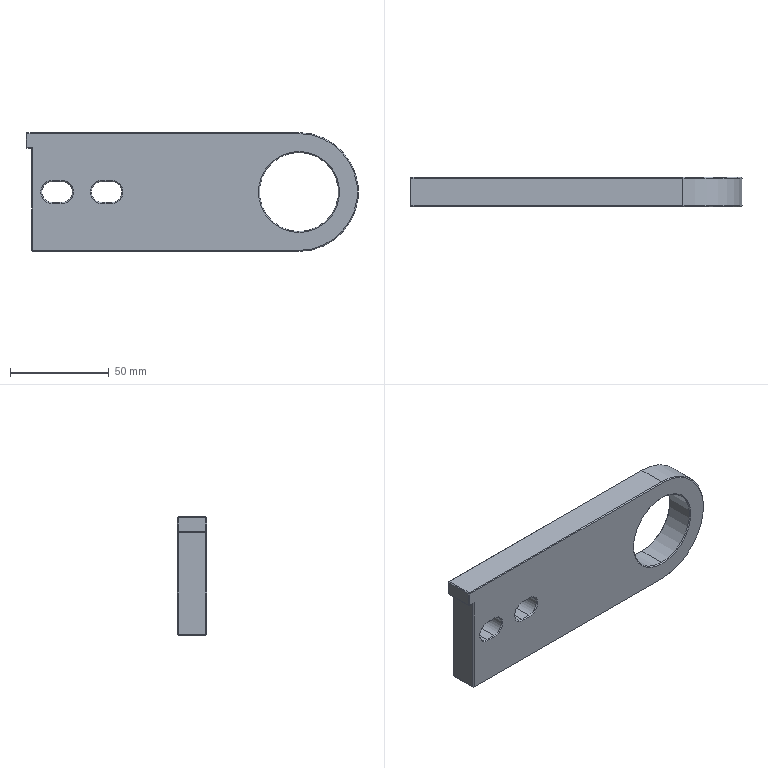Part | SolidWorks | features Chamfer 1, Extrusion 1, ICE 1 | 1 solid | 59 faces | box 168 x 15 x 60 mm | volume 119877 mm3 | plane 38 | cone 14 | cylinder 7 | commonest cylinder face diameters 10.5 x4 40 x2 60 x1
STEP:
#1=CARTESIAN_POINT('',(0.,0.5,20.));
#2=VERTEX_POINT('',#1);
#3=CARTESIAN_POINT('',(0.,0.5,-20.));
#4=VERTEX_POINT('',#3);
#5=CARTESIAN_POINT('',(0.,0.5,0.));
#6=DIRECTION('',(0.,-1.,0.));
#7=DIRECTION('',(0.,0.,1.));
#8=AXIS2_PLACEMENT_3D('',#5,#6,#7);
#9=CIRCLE('',#8,20.);
#10=EDGE_CURVE('',#2,#4,#9,.T.);
#11=ORIENTED_EDGE('',*,*,#10,.F.);
#12=CARTESIAN_POINT('',(0.,0.,20.5));
#13=VERTEX_POINT('',#12);
#14=CARTESIAN_POINT('',(0.,0.,20.5));
#15=DIRECTION('',(0.,-0.7071,0.7071));
#16=VECTOR('',#15,1000.);
#17=LINE('',#14,#16);
#18=EDGE_CURVE('',#2,#13,#17,.T.);
#19=ORIENTED_EDGE('',*,*,#18,.T.);
#20=CARTESIAN_POINT('',(0.,0.,-20.5));
#21=VERTEX_POINT('',#20);
#22=CARTESIAN_POINT('',(0.,0.,0.));
#23=DIRECTION('',(0.,1.,0.));
#24=DIRECTION('',(0.,0.,1.));
#25=AXIS2_PLACEMENT_3D('',#22,#23,#24);
#26=CIRCLE('',#25,20.5);
#27=EDGE_CURVE('',#21,#13,#26,.T.);
#28=ORIENTED_EDGE('',*,*,#27,.F.);
#29=CARTESIAN_POINT('',(0.,0.,-20.5));
#30=DIRECTION('',(0.,-0.7071,-0.7071));
#31=VECTOR('',#30,1000.);
#32=LINE('',#29,#31);
#33=EDGE_CURVE('',#4,#21,#32,.T.);
#34=ORIENTED_EDGE('',*,*,#33,.F.);
#35=EDGE_LOOP('',(#11,#19,#28,#34));
#36=FACE_OUTER_BOUND('',#35,.T.);
#37=CARTESIAN_POINT('',(0.,0.,0.));
#38=DIRECTION('',(0.,-1.,0.));
#39=DIRECTION('',(0.,0.,-1.));
#40=AXIS2_PLACEMENT_3D('',#37,#38,#39);
#41=CONICAL_SURFACE('',#40,20.5,0.7854);
#42=ADVANCED_FACE('',(#36),#41,.F.);
#43=CARTESIAN_POINT('',(0.,14.5,-20.));
#44=VERTEX_POINT('',#43);
#45=CARTESIAN_POINT('',(0.,14.5,20.));
#46=VERTEX_POINT('',#45);
#47=CARTESIAN_POINT('',(0.,14.5,0.));
#48=DIRECTION('',(0.,1.,0.));
#49=DIRECTION('',(0.,0.,1.));
#50=AXIS2_PLACEMENT_3D('',#47,#48,#49);
#51=CIRCLE('',#50,20.);
#52=EDGE_CURVE('',#44,#46,#51,.T.);
#53=ORIENTED_EDGE('',*,*,#52,.F.);
#54=CARTESIAN_POINT('',(0.,15.,-20.5));
#55=VERTEX_POINT('',#54);
#56=CARTESIAN_POINT('',(0.,14.5,-20.));
#57=DIRECTION('',(0.,0.7071,-0.7071));
#58=VECTOR('',#57,1000.);
#59=LINE('',#56,#58);
#60=EDGE_CURVE('',#44,#55,#59,.T.);
#61=ORIENTED_EDGE('',*,*,#60,.T.);
#62=CARTESIAN_POINT('',(0.,15.,20.5));
#63=VERTEX_POINT('',#62);
#64=CARTESIAN_POINT('',(0.,15.,0.));
#65=DIRECTION('',(0.,-1.,0.));
#66=DIRECTION('',(0.,0.,1.));
#67=AXIS2_PLACEMENT_3D('',#64,#65,#66);
#68=CIRCLE('',#67,20.5);
#69=EDGE_CURVE('',#63,#55,#68,.T.);
#70=ORIENTED_EDGE('',*,*,#69,.F.);
#71=CARTESIAN_POINT('',(0.,14.5,20.));
#72=DIRECTION('',(0.,0.7071,0.7071));
#73=VECTOR('',#72,1000.);
#74=LINE('',#71,#73);
#75=EDGE_CURVE('',#46,#63,#74,.T.);
#76=ORIENTED_EDGE('',*,*,#75,.F.);
#77=EDGE_LOOP('',(#53,#61,#70,#76));
#78=FACE_OUTER_BOUND('',#77,.T.);
#79=CARTESIAN_POINT('',(0.,14.5,0.));
#80=DIRECTION('',(0.,1.,0.));
#81=DIRECTION('',(0.,0.,1.));
#82=AXIS2_PLACEMENT_3D('',#79,#80,#81);
#83=CONICAL_SURFACE('',#82,20.,0.7854);
#84=ADVANCED_FACE('',(#78),#83,.F.);
#85=ORIENTED_EDGE('',*,*,#52,.T.);
#86=CARTESIAN_POINT('',(0.,15.,20.));
#87=DIRECTION('',(0.,-1.,0.));
#88=VECTOR('',#87,1000.);
#89=LINE('',#86,#88);
#90=EDGE_CURVE('',#46,#2,#89,.T.);
#91=ORIENTED_EDGE('',*,*,#90,.T.);
#92=ORIENTED_EDGE('',*,*,#10,.T.);
#93=CARTESIAN_POINT('',(0.,15.,-20.));
#94=DIRECTION('',(0.,-1.,0.));
#95=VECTOR('',#94,1000.);
#96=LINE('',#93,#95);
#97=EDGE_CURVE('',#44,#4,#96,.T.);
#98=ORIENTED_EDGE('',*,*,#97,.F.);
#99=EDGE_LOOP('',(#85,#91,#92,#98));
#100=FACE_OUTER_BOUND('',#99,.T.);
#101=CARTESIAN_POINT('',(0.,15.,0.));
#102=DIRECTION('',(0.,-1.,0.));
#103=DIRECTION('',(0.,0.,-1.));
#104=AXIS2_PLACEMENT_3D('',#101,#102,#103);
#105=CYLINDRICAL_SURFACE('',#104,20.);
#106=ADVANCED_FACE('',(#100),#105,.F.);
#107=CARTESIAN_POINT('',(-135.,14.5,22.));
#108=VERTEX_POINT('',#107);
#109=CARTESIAN_POINT('',(-135.,0.5,22.));
#110=VERTEX_POINT('',#109);
#111=CARTESIAN_POINT('',(-135.,15.,22.));
#112=DIRECTION('',(0.,-1.,0.));
#113=VECTOR('',#112,1000.);
#114=LINE('',#111,#113);
#115=EDGE_CURVE('',#108,#110,#114,.T.);
#116=ORIENTED_EDGE('',*,*,#115,.F.);
#117=CARTESIAN_POINT('',(-135.,14.5,-29.5));
#118=VERTEX_POINT('',#117);
#119=CARTESIAN_POINT('',(-135.,14.5,-30.));
#120=DIRECTION('',(0.,0.,-1.));
#121=VECTOR('',#120,1000.);
#122=LINE('',#119,#121);
#123=EDGE_CURVE('',#108,#118,#122,.T.);
#124=ORIENTED_EDGE('',*,*,#123,.T.);
#125=CARTESIAN_POINT('',(-135.,0.5,-29.5));
#126=VERTEX_POINT('',#125);
#127=CARTESIAN_POINT('',(-135.,15.,-29.5));
#128=DIRECTION('',(0.,-1.,0.));
#129=VECTOR('',#128,1000.);
#130=LINE('',#127,#129);
#131=EDGE_CURVE('',#118,#126,#130,.T.);
#132=ORIENTED_EDGE('',*,*,#131,.T.);
#133=CARTESIAN_POINT('',(-135.,0.5,-30.));
#134=DIRECTION('',(0.,0.,1.));
#135=VECTOR('',#134,1000.);
#136=LINE('',#133,#135);
#137=EDGE_CURVE('',#126,#110,#136,.T.);
#138=ORIENTED_EDGE('',*,*,#137,.T.);
#139=EDGE_LOOP('',(#116,#124,#132,#138));
#140=FACE_OUTER_BOUND('',#139,.T.);
#141=CARTESIAN_POINT('',(-135.,15.,-30.));
#142=DIRECTION('',(1.,0.,0.));
#143=DIRECTION('',(0.,0.,-1.));
#144=AXIS2_PLACEMENT_3D('',#141,#142,#143);
#145=PLANE('',#144);
#146=ADVANCED_FACE('',(#140),#145,.F.);
#147=ORIENTED_EDGE('',*,*,#69,.T.);
#148=CARTESIAN_POINT('',(0.,15.,0.));
#149=DIRECTION('',(0.,-1.,0.));
#150=DIRECTION('',(0.,0.,1.));
#151=AXIS2_PLACEMENT_3D('',#148,#149,#150);
#152=CIRCLE('',#151,20.5);
#153=EDGE_CURVE('',#55,#63,#152,.T.);
#154=ORIENTED_EDGE('',*,*,#153,.T.);
#155=EDGE_LOOP('',(#147,#154));
#156=FACE_BOUND('',#155,.T.);
#157=CARTESIAN_POINT('',(-124.75,15.,5.75));
#158=VERTEX_POINT('',#157);
#159=CARTESIAN_POINT('',(-124.75,15.,-5.75));
#160=VERTEX_POINT('',#159);
#161=CARTESIAN_POINT('',(-124.75,15.,0.));
#162=DIRECTION('',(0.,-1.,0.));
#163=DIRECTION('',(0.,0.,1.));
#164=AXIS2_PLACEMENT_3D('',#161,#162,#163);
#165=CIRCLE('',#164,5.75);
#166=EDGE_CURVE('',#158,#160,#165,.T.);
#167=ORIENTED_EDGE('',*,*,#166,.T.);
#168=CARTESIAN_POINT('',(-119.75,15.,-5.75));
#169=VERTEX_POINT('',#168);
#170=CARTESIAN_POINT('',(0.,15.,-5.75));
#171=DIRECTION('',(1.,0.,0.));
#172=VECTOR('',#171,1000.);
#173=LINE('',#170,#172);
#174=EDGE_CURVE('',#160,#169,#173,.T.);
#175=ORIENTED_EDGE('',*,*,#174,.T.);
#176=CARTESIAN_POINT('',(-119.75,15.,5.75));
#177=VERTEX_POINT('',#176);
#178=CARTESIAN_POINT('',(-119.75,15.,0.));
#179=DIRECTION('',(0.,-1.,0.));
#180=DIRECTION('',(0.,0.,1.));
#181=AXIS2_PLACEMENT_3D('',#178,#179,#180);
#182=CIRCLE('',#181,5.75);
#183=EDGE_CURVE('',#169,#177,#182,.T.);
#184=ORIENTED_EDGE('',*,*,#183,.T.);
#185=CARTESIAN_POINT('',(0.,15.,5.75));
#186=DIRECTION('',(-1.,0.,0.));
#187=VECTOR('',#186,1000.);
#188=LINE('',#185,#187);
#189=EDGE_CURVE('',#177,#158,#188,.T.);
#190=ORIENTED_EDGE('',*,*,#189,.T.);
#191=EDGE_LOOP('',(#167,#175,#184,#190));
#192=FACE_BOUND('',#191,.T.);
#193=CARTESIAN_POINT('',(-99.75,15.,5.75));
#194=VERTEX_POINT('',#193);
#195=CARTESIAN_POINT('',(-99.75,15.,-5.75));
#196=VERTEX_POINT('',#195);
#197=CARTESIAN_POINT('',(-99.75,15.,0.));
#198=DIRECTION('',(0.,-1.,0.));
#199=DIRECTION('',(0.,0.,1.));
#200=AXIS2_PLACEMENT_3D('',#197,#198,#199);
#201=CIRCLE('',#200,5.75);
#202=EDGE_CURVE('',#194,#196,#201,.T.);
#203=ORIENTED_EDGE('',*,*,#202,.T.);
#204=CARTESIAN_POINT('',(-94.75,15.,-5.75));
#205=VERTEX_POINT('',#204);
#206=CARTESIAN_POINT('',(0.,15.,-5.75));
#207=DIRECTION('',(1.,0.,0.));
#208=VECTOR('',#207,1000.);
#209=LINE('',#206,#208);
#210=EDGE_CURVE('',#196,#205,#209,.T.);
#211=ORIENTED_EDGE('',*,*,#210,.T.);
#212=CARTESIAN_POINT('',(-94.75,15.,5.75));
#213=VERTEX_POINT('',#212);
#214=CARTESIAN_POINT('',(-94.75,15.,0.));
#215=DIRECTION('',(0.,-1.,0.));
#216=DIRECTION('',(0.,0.,1.));
#217=AXIS2_PLACEMENT_3D('',#214,#215,#216);
#218=CIRCLE('',#217,5.75);
#219=EDGE_CURVE('',#205,#213,#218,.T.);
#220=ORIENTED_EDGE('',*,*,#219,.T.);
#221=CARTESIAN_POINT('',(0.,15.,5.75));
#222=DIRECTION('',(-1.,0.,0.));
#223=VECTOR('',#222,1000.);
#224=LINE('',#221,#223);
#225=EDGE_CURVE('',#213,#194,#224,.T.);
#226=ORIENTED_EDGE('',*,*,#225,.T.);
#227=EDGE_LOOP('',(#203,#211,#220,#226));
#228=FACE_BOUND('',#227,.T.);
#229=CARTESIAN_POINT('',(0.,15.,-29.5));
#230=VERTEX_POINT('',#229);
#231=CARTESIAN_POINT('',(-134.5,15.,-29.5));
#232=VERTEX_POINT('',#231);
#233=CARTESIAN_POINT('',(-135.,15.,-29.5));
#234=DIRECTION('',(-1.,0.,0.));
#235=VECTOR('',#234,1000.);
#236=LINE('',#233,#235);
#237=EDGE_CURVE('',#230,#232,#236,.T.);
#238=ORIENTED_EDGE('',*,*,#237,.T.);
#239=CARTESIAN_POINT('',(-134.5,15.,22.5));
#240=VERTEX_POINT('',#239);
#241=CARTESIAN_POINT('',(-134.5,15.,22.));
#242=DIRECTION('',(0.,0.,1.));
#243=VECTOR('',#242,1000.);
#244=LINE('',#241,#243);
#245=EDGE_CURVE('',#232,#240,#244,.T.);
#246=ORIENTED_EDGE('',*,*,#245,.T.);
#247=CARTESIAN_POINT('',(-137.5,15.,22.5));
#248=VERTEX_POINT('',#247);
#249=CARTESIAN_POINT('',(0.,15.,22.5));
#250=DIRECTION('',(-1.,0.,0.));
#251=VECTOR('',#250,1000.);
#252=LINE('',#249,#251);
#253=EDGE_CURVE('',#240,#248,#252,.T.);
#254=ORIENTED_EDGE('',*,*,#253,.T.);
#255=CARTESIAN_POINT('',(-137.5,15.,29.5));
#256=VERTEX_POINT('',#255);
#257=CARTESIAN_POINT('',(-137.5,15.,0.));
#258=DIRECTION('',(0.,0.,1.));
#259=VECTOR('',#258,1000.);
#260=LINE('',#257,#259);
#261=EDGE_CURVE('',#248,#256,#260,.T.);
#262=ORIENTED_EDGE('',*,*,#261,.T.);
#263=CARTESIAN_POINT('',(0.,15.,29.5));
#264=VERTEX_POINT('',#263);
#265=CARTESIAN_POINT('',(0.,15.,29.5));
#266=DIRECTION('',(1.,0.,0.));
#267=VECTOR('',#266,1000.);
#268=LINE('',#265,#267);
#269=EDGE_CURVE('',#256,#264,#268,.T.);
#270=ORIENTED_EDGE('',*,*,#269,.T.);
#271=CARTESIAN_POINT('',(0.,15.,0.));
#272=DIRECTION('',(0.,1.,0.));
#273=DIRECTION('',(0.,0.,1.));
#274=AXIS2_PLACEMENT_3D('',#271,#272,#273);
#275=CIRCLE('',#274,29.5);
#276=EDGE_CURVE('',#264,#230,#275,.T.);
#277=ORIENTED_EDGE('',*,*,#276,.T.);
#278=EDGE_LOOP('',(#238,#246,#254,#262,#270,#277));
#279=FACE_OUTER_BOUND('',#278,.T.);
#280=CARTESIAN_POINT('',(0.,15.,0.));
#281=DIRECTION('',(0.,1.,0.));
#282=DIRECTION('',(0.,0.,1.));
#283=AXIS2_PLACEMENT_3D('',#280,#281,#282);
#284=PLANE('',#283);
#285=ADVANCED_FACE('',(#156,#192,#228,#279),#284,.T.);
#286=ORIENTED_EDGE('',*,*,#27,.T.);
#287=CARTESIAN_POINT('',(0.,0.,0.));
#288=DIRECTION('',(0.,1.,0.));
#289=DIRECTION('',(0.,0.,1.));
#290=AXIS2_PLACEMENT_3D('',#287,#288,#289);
#291=CIRCLE('',#290,20.5);
#292=EDGE_CURVE('',#13,#21,#291,.T.);
#293=ORIENTED_EDGE('',*,*,#292,.T.);
#294=EDGE_LOOP('',(#286,#293));
#295=FACE_BOUND('',#294,.T.);
#296=CARTESIAN_POINT('',(-119.75,0.,5.75));
#297=VERTEX_POINT('',#296);
#298=CARTESIAN_POINT('',(-119.75,0.,-5.75));
#299=VERTEX_POINT('',#298);
#300=CARTESIAN_POINT('',(-119.75,0.,0.));
#301=DIRECTION('',(0.,1.,0.));
#302=DIRECTION('',(0.,0.,1.));
#303=AXIS2_PLACEMENT_3D('',#300,#301,#302);
#304=CIRCLE('',#303,5.75);
#305=EDGE_CURVE('',#297,#299,#304,.T.);
#306=ORIENTED_EDGE('',*,*,#305,.T.);
#307=CARTESIAN_POINT('',(-124.75,0.,-5.75));
#308=VERTEX_POINT('',#307);
#309=CARTESIAN_POINT('',(-124.75,0.,-5.75));
#310=DIRECTION('',(-1.,0.,0.));
#311=VECTOR('',#310,1000.);
#312=LINE('',#309,#311);
#313=EDGE_CURVE('',#299,#308,#312,.T.);
#314=ORIENTED_EDGE('',*,*,#313,.T.);
#315=CARTESIAN_POINT('',(-124.75,0.,5.75));
#316=VERTEX_POINT('',#315);
#317=CARTESIAN_POINT('',(-124.75,0.,0.));
#318=DIRECTION('',(0.,1.,0.));
#319=DIRECTION('',(0.,0.,1.));
#320=AXIS2_PLACEMENT_3D('',#317,#318,#319);
#321=CIRCLE('',#320,5.75);
#322=EDGE_CURVE('',#308,#316,#321,.T.);
#323=ORIENTED_EDGE('',*,*,#322,.T.);
#324=CARTESIAN_POINT('',(-119.75,0.,5.75));
#325=DIRECTION('',(1.,0.,0.));
#326=VECTOR('',#325,1000.);
#327=LINE('',#324,#326);
#328=EDGE_CURVE('',#316,#297,#327,.T.);
#329=ORIENTED_EDGE('',*,*,#328,.T.);
#330=EDGE_LOOP('',(#306,#314,#323,#329));
#331=FACE_BOUND('',#330,.T.);
#332=CARTESIAN_POINT('',(-94.75,0.,5.75));
#333=VERTEX_POINT('',#332);
#334=CARTESIAN_POINT('',(-94.75,0.,-5.75));
#335=VERTEX_POINT('',#334);
#336=CARTESIAN_POINT('',(-94.75,0.,0.));
#337=DIRECTION('',(0.,1.,0.));
#338=DIRECTION('',(0.,0.,1.));
#339=AXIS2_PLACEMENT_3D('',#336,#337,#338);
#340=CIRCLE('',#339,5.75);
#341=EDGE_CURVE('',#333,#335,#340,.T.);
#342=ORIENTED_EDGE('',*,*,#341,.T.);
#343=CARTESIAN_POINT('',(-99.75,0.,-5.75));
#344=VERTEX_POINT('',#343);
#345=CARTESIAN_POINT('',(-99.75,0.,-5.75));
#346=DIRECTION('',(-1.,0.,0.));
#347=VECTOR('',#346,1000.);
#348=LINE('',#345,#347);
#349=EDGE_CURVE('',#335,#344,#348,.T.);
#350=ORIENTED_EDGE('',*,*,#349,.T.);
#351=CARTESIAN_POINT('',(-99.75,0.,5.75));
#352=VERTEX_POINT('',#351);
#353=CARTESIAN_POINT('',(-99.75,0.,0.));
#354=DIRECTION('',(0.,1.,0.));
#355=DIRECTION('',(0.,0.,1.));
#356=AXIS2_PLACEMENT_3D('',#353,#354,#355);
#357=CIRCLE('',#356,5.75);
#358=EDGE_CURVE('',#344,#352,#357,.T.);
#359=ORIENTED_EDGE('',*,*,#358,.T.);
#360=CARTESIAN_POINT('',(-94.75,0.,5.75));
#361=DIRECTION('',(1.,0.,0.));
#362=VECTOR('',#361,1000.);
#363=LINE('',#360,#362);
#364=EDGE_CURVE('',#352,#333,#363,.T.);
#365=ORIENTED_EDGE('',*,*,#364,.T.);
#366=EDGE_LOOP('',(#342,#350,#359,#365));
#367=FACE_BOUND('',#366,.T.);
#368=CARTESIAN_POINT('',(-137.5,0.,22.5));
#369=VERTEX_POINT('',#368);
#370=CARTESIAN_POINT('',(-134.5,0.,22.5));
#371=VERTEX_POINT('',#370);
#372=CARTESIAN_POINT('',(-135.,0.,22.5));
#373=DIRECTION('',(1.,0.,0.));
#374=VECTOR('',#373,1000.);
#375=LINE('',#372,#374);
#376=EDGE_CURVE('',#369,#371,#375,.T.);
#377=ORIENTED_EDGE('',*,*,#376,.T.);
#378=CARTESIAN_POINT('',(-134.5,0.,-29.5));
#379=VERTEX_POINT('',#378);
#380=CARTESIAN_POINT('',(-134.5,0.,0.));
#381=DIRECTION('',(0.,0.,-1.));
#382=VECTOR('',#381,1000.);
#383=LINE('',#380,#382);
#384=EDGE_CURVE('',#371,#379,#383,.T.);
#385=ORIENTED_EDGE('',*,*,#384,.T.);
#386=CARTESIAN_POINT('',(0.,0.,-29.5));
#387=VERTEX_POINT('',#386);
#388=CARTESIAN_POINT('',(0.,0.,-29.5));
#389=DIRECTION('',(1.,0.,0.));
#390=VECTOR('',#389,1000.);
#391=LINE('',#388,#390);
#392=EDGE_CURVE('',#379,#387,#391,.T.);
#393=ORIENTED_EDGE('',*,*,#392,.T.);
#394=CARTESIAN_POINT('',(0.,0.,29.5));
#395=VERTEX_POINT('',#394);
#396=CARTESIAN_POINT('',(0.,0.,0.));
#397=DIRECTION('',(0.,-1.,0.));
#398=DIRECTION('',(0.,0.,1.));
#399=AXIS2_PLACEMENT_3D('',#396,#397,#398);
#400=CIRCLE('',#399,29.5);
#401=EDGE_CURVE('',#387,#395,#400,.T.);
#402=ORIENTED_EDGE('',*,*,#401,.T.);
#403=CARTESIAN_POINT('',(-137.5,0.,29.5));
#404=VERTEX_POINT('',#403);
#405=CARTESIAN_POINT('',(0.,0.,29.5));
#406=DIRECTION('',(-1.,0.,0.));
#407=VECTOR('',#406,1000.);
#408=LINE('',#405,#407);
#409=EDGE_CURVE('',#395,#404,#408,.T.);
#410=ORIENTED_EDGE('',*,*,#409,.T.);
#411=CARTESIAN_POINT('',(-137.5,0.,22.));
#412=DIRECTION('',(0.,0.,-1.));
#413=VECTOR('',#412,1000.);
#414=LINE('',#411,#413);
#415=EDGE_CURVE('',#404,#369,#414,.T.);
#416=ORIENTED_EDGE('',*,*,#415,.T.);
#417=EDGE_LOOP('',(#377,#385,#393,#402,#410,#416));
#418=FACE_OUTER_BOUND('',#417,.T.);
#419=CARTESIAN_POINT('',(0.,0.,0.));
#420=DIRECTION('',(0.,1.,0.));
#421=DIRECTION('',(0.,0.,1.));
#422=AXIS2_PLACEMENT_3D('',#419,#420,#421);
#423=PLANE('',#422);
#424=ADVANCED_FACE('',(#295,#331,#367,#418),#423,.F.);
#425=CARTESIAN_POINT('',(0.,14.5,30.));
#426=VERTEX_POINT('',#425);
#427=CARTESIAN_POINT('',(0.,0.5,30.));
#428=VERTEX_POINT('',#427);
#429=CARTESIAN_POINT('',(0.,15.,30.));
#430=DIRECTION('',(0.,-1.,0.));
#431=VECTOR('',#430,1000.);
#432=LINE('',#429,#431);
#433=EDGE_CURVE('',#426,#428,#432,.T.);
#434=ORIENTED_EDGE('',*,*,#433,.F.);
#435=CARTESIAN_POINT('',(-137.5,14.5,30.));
#436=VERTEX_POINT('',#435);
#437=CARTESIAN_POINT('',(-138.,14.5,30.));
#438=DIRECTION('',(-1.,0.,0.));
#439=VECTOR('',#438,1000.);
#440=LINE('',#437,#439);
#441=EDGE_CURVE('',#426,#436,#440,.T.);
#442=ORIENTED_EDGE('',*,*,#441,.T.);
#443=CARTESIAN_POINT('',(-137.5,0.5,30.));
#444=VERTEX_POINT('',#443);
#445=CARTESIAN_POINT('',(-137.5,0.,30.));
#446=DIRECTION('',(0.,-1.,0.));
#447=VECTOR('',#446,1000.);
#448=LINE('',#445,#447);
#449=EDGE_CURVE('',#436,#444,#448,.T.);
#450=ORIENTED_EDGE('',*,*,#449,.T.);
#451=CARTESIAN_POINT('',(-135.,0.5,30.));
#452=DIRECTION('',(1.,0.,0.));
#453=VECTOR('',#452,1000.);
#454=LINE('',#451,#453);
#455=EDGE_CURVE('',#444,#428,#454,.T.);
#456=ORIENTED_EDGE('',*,*,#455,.T.);
#457=EDGE_LOOP('',(#434,#442,#450,#456));
#458=FACE_OUTER_BOUND('',#457,.T.);
#459=CARTESIAN_POINT('',(-135.,15.,30.));
#460=DIRECTION('',(0.,0.,-1.));
#461=DIRECTION('',(-1.,0.,0.));
#462=AXIS2_PLACEMENT_3D('',#459,#460,#461);
#463=PLANE('',#462);
#464=ADVANCED_FACE('',(#458),#463,.F.);
#465=CARTESIAN_POINT('',(0.,14.5,-30.));
#466=VERTEX_POINT('',#465);
#467=CARTESIAN_POINT('',(0.,0.5,-30.));
#468=VERTEX_POINT('',#467);
#469=CARTESIAN_POINT('',(0.,15.,-30.));
#470=DIRECTION('',(0.,-1.,0.));
#471=VECTOR('',#470,1000.);
#472=LINE('',#469,#471);
#473=EDGE_CURVE('',#466,#468,#472,.T.);
#474=ORIENTED_EDGE('',*,*,#473,.F.);
#475=CARTESIAN_POINT('',(0.,14.5,0.));
#476=DIRECTION('',(0.,-1.,0.));
#477=DIRECTION('',(0.,0.,1.));
#478=AXIS2_PLACEMENT_3D('',#475,#476,#477);
#479=CIRCLE('',#478,30.);
#480=EDGE_CURVE('',#466,#426,#479,.T.);
#481=ORIENTED_EDGE('',*,*,#480,.T.);
#482=ORIENTED_EDGE('',*,*,#433,.T.);
#483=CARTESIAN_POINT('',(0.,0.5,0.));
#484=DIRECTION('',(0.,1.,0.));
#485=DIRECTION('',(0.,0.,1.));
#486=AXIS2_PLACEMENT_3D('',#483,#484,#485);
#487=CIRCLE('',#486,30.);
#488=EDGE_CURVE('',#428,#468,#487,.T.);
#489=ORIENTED_EDGE('',*,*,#488,.T.);
#490=EDGE_LOOP('',(#474,#481,#482,#489));
#491=FACE_OUTER_BOUND('',#490,.T.);
#492=CARTESIAN_POINT('',(0.,15.,0.));
#493=DIRECTION('',(0.,-1.,0.));
#494=DIRECTION('',(0.,0.,-1.));
#495=AXIS2_PLACEMENT_3D('',#492,#493,#494);
#496=CYLINDRICAL_SURFACE('',#495,30.);
#497=ADVANCED_FACE('',(#491),#496,.T.);
#498=CARTESIAN_POINT('',(-134.5,0.5,-30.));
#499=VERTEX_POINT('',#498);
#500=CARTESIAN_POINT('',(-134.5,14.5,-30.));
#501=VERTEX_POINT('',#500);
#502=CARTESIAN_POINT('',(-134.5,15.,-30.));
#503=DIRECTION('',(0.,1.,0.));
#504=VECTOR('',#503,1000.);
#505=LINE('',#502,#504);
#506=EDGE_CURVE('',#499,#501,#505,.T.);
#507=ORIENTED_EDGE('',*,*,#506,.T.);
#508=CARTESIAN_POINT('',(0.,14.5,-30.));
#509=DIRECTION('',(1.,0.,0.));
#510=VECTOR('',#509,1000.);
#511=LINE('',#508,#510);
#512=EDGE_CURVE('',#501,#466,#511,.T.);
#513=ORIENTED_EDGE('',*,*,#512,.T.);
#514=ORIENTED_EDGE('',*,*,#473,.T.);
#515=CARTESIAN_POINT('',(-135.,0.5,-30.));
#516=DIRECTION('',(-1.,0.,0.));
#517=VECTOR('',#516,1000.);
#518=LINE('',#515,#517);
#519=EDGE_CURVE('',#468,#499,#518,.T.);
#520=ORIENTED_EDGE('',*,*,#519,.T.);
#521=EDGE_LOOP('',(#507,#513,#514,#520));
#522=FACE_OUTER_BOUND('',#521,.T.);
#523=CARTESIAN_POINT('',(-135.,15.,-30.));
#524=DIRECTION('',(0.,0.,1.));
#525=DIRECTION('',(1.,0.,0.));
#526=AXIS2_PLACEMENT_3D('',#523,#524,#525);
#527=PLANE('',#526);
#528=ADVANCED_FACE('',(#522),#527,.F.);
#529=ORIENTED_EDGE('',*,*,#90,.F.);
#530=CARTESIAN_POINT('',(0.,14.5,0.));
#531=DIRECTION('',(0.,1.,0.));
#532=DIRECTION('',(0.,0.,1.));
#533=AXIS2_PLACEMENT_3D('',#530,#531,#532);
#534=CIRCLE('',#533,20.);
#535=EDGE_CURVE('',#46,#44,#534,.T.);
#536=ORIENTED_EDGE('',*,*,#535,.T.);
#537=ORIENTED_EDGE('',*,*,#97,.T.);
#538=CARTESIAN_POINT('',(0.,0.5,0.));
#539=DIRECTION('',(0.,-1.,0.));
#540=DIRECTION('',(0.,0.,1.));
#541=AXIS2_PLACEMENT_3D('',#538,#539,#540);
#542=CIRCLE('',#541,20.);
#543=EDGE_CURVE('',#4,#2,#542,.T.);
#544=ORIENTED_EDGE('',*,*,#543,.T.);
#545=EDGE_LOOP('',(#529,#536,#537,#544));
#546=FACE_OUTER_BOUND('',#545,.T.);
#547=CARTESIAN_POINT('',(0.,15.,0.));
#548=DIRECTION('',(0.,-1.,0.));
#549=DIRECTION('',(0.,0.,-1.));
#550=AXIS2_PLACEMENT_3D('',#547,#548,#549);
#551=CYLINDRICAL_SURFACE('',#550,20.);
#552=ADVANCED_FACE('',(#546),#551,.F.);
#553=CARTESIAN_POINT('',(-124.75,14.5,-5.25));
#554=VERTEX_POINT('',#553);
#555=CARTESIAN_POINT('',(-124.75,0.5,-5.25));
#556=VERTEX_POINT('',#555);
#557=CARTESIAN_POINT('',(-124.75,15.,-5.25));
#558=DIRECTION('',(0.,-1.,0.));
#559=VECTOR('',#558,1000.);
#560=LINE('',#557,#559);
#561=EDGE_CURVE('',#554,#556,#560,.T.);
#562=ORIENTED_EDGE('',*,*,#561,.F.);
#563=CARTESIAN_POINT('',(-124.75,14.5,5.25));
#564=VERTEX_POINT('',#563);
#565=CARTESIAN_POINT('',(-124.75,14.5,0.));
#566=DIRECTION('',(0.,1.,0.));
#567=DIRECTION('',(0.,0.,1.));
#568=AXIS2_PLACEMENT_3D('',#565,#566,#567);
#569=CIRCLE('',#568,5.25);
#570=EDGE_CURVE('',#554,#564,#569,.T.);
#571=ORIENTED_EDGE('',*,*,#570,.T.);
#572=CARTESIAN_POINT('',(-124.75,0.5,5.25));
#573=VERTEX_POINT('',#572);
#574=CARTESIAN_POINT('',(-124.75,15.,5.25));
#575=DIRECTION('',(0.,-1.,0.));
#576=VECTOR('',#575,1000.);
#577=LINE('',#574,#576);
#578=EDGE_CURVE('',#564,#573,#577,.T.);
#579=ORIENTED_EDGE('',*,*,#578,.T.);
#580=CARTESIAN_POINT('',(-124.75,0.5,0.));
#581=DIRECTION('',(0.,-1.,0.));
#582=DIRECTION('',(0.,0.,1.));
#583=AXIS2_PLACEMENT_3D('',#580,#581,#582);
#584=CIRCLE('',#583,5.25);
#585=EDGE_CURVE('',#573,#556,#584,.T.);
#586=ORIENTED_EDGE('',*,*,#585,.T.);
#587=EDGE_LOOP('',(#562,#571,#579,#586));
#588=FACE_OUTER_BOUND('',#587,.T.);
#589=CARTESIAN_POINT('',(-124.75,15.,0.));
#590=DIRECTION('',(0.,-1.,0.));
#591=DIRECTION('',(0.,0.,-1.));
#592=AXIS2_PLACEMENT_3D('',#589,#590,#591);
#593=CYLINDRICAL_SURFACE('',#592,5.25);
#594=ADVANCED_FACE('',(#588),#593,.F.);
#595=ORIENTED_EDGE('',*,*,#578,.F.);
#596=CARTESIAN_POINT('',(-119.75,14.5,5.25));
#597=VERTEX_POINT('',#596);
#598=CARTESIAN_POINT('',(-124.75,14.5,5.25));
#599=DIRECTION('',(1.,0.,0.));
#600=VECTOR('',#599,1000.);
#601=LINE('',#598,#600);
#602=EDGE_CURVE('',#564,#597,#601,.T.);
#603=ORIENTED_EDGE('',*,*,#602,.T.);
#604=CARTESIAN_POINT('',(-119.75,0.5,5.25));
#605=VERTEX_POINT('',#604);
#606=CARTESIAN_POINT('',(-119.75,15.,5.25));
#607=DIRECTION('',(0.,-1.,0.));
#608=VECTOR('',#607,1000.);
#609=LINE('',#606,#608);
#610=EDGE_CURVE('',#597,#605,#609,.T.);
#611=ORIENTED_EDGE('',*,*,#610,.T.);
#612=CARTESIAN_POINT('',(-124.75,0.5,5.25));
#613=DIRECTION('',(-1.,0.,0.));
#614=VECTOR('',#613,1000.);
#615=LINE('',#612,#614);
#616=EDGE_CURVE('',#605,#573,#615,.T.);
#617=ORIENTED_EDGE('',*,*,#616,.T.);
#618=EDGE_LOOP('',(#595,#603,#611,#617));
#619=FACE_OUTER_BOUND('',#618,.T.);
#620=CARTESIAN_POINT('',(-124.75,15.,5.25));
#621=DIRECTION('',(0.,0.,-1.));
#622=DIRECTION('',(-1.,0.,0.));
#623=AXIS2_PLACEMENT_3D('',#620,#621,#622);
#624=PLANE('',#623);
#625=ADVANCED_FACE('',(#619),#624,.T.);
#626=ORIENTED_EDGE('',*,*,#610,.F.);
#627=CARTESIAN_POINT('',(-119.75,14.5,-5.25));
#628=VERTEX_POINT('',#627);
#629=CARTESIAN_POINT('',(-119.75,14.5,0.));
#630=DIRECTION('',(0.,1.,0.));
#631=DIRECTION('',(0.,0.,1.));
#632=AXIS2_PLACEMENT_3D('',#629,#630,#631);
#633=CIRCLE('',#632,5.25);
#634=EDGE_CURVE('',#597,#628,#633,.T.);
#635=ORIENTED_EDGE('',*,*,#634,.T.);
#636=CARTESIAN_POINT('',(-119.75,0.5,-5.25));
#637=VERTEX_POINT('',#636);
#638=CARTESIAN_POINT('',(-119.75,15.,-5.25));
#639=DIRECTION('',(0.,-1.,0.));
#640=VECTOR('',#639,1000.);
#641=LINE('',#638,#640);
#642=EDGE_CURVE('',#628,#637,#641,.T.);
#643=ORIENTED_EDGE('',*,*,#642,.T.);
#644=CARTESIAN_POINT('',(-119.75,0.5,0.));
#645=DIRECTION('',(0.,-1.,0.));
#646=DIRECTION('',(0.,0.,1.));
#647=AXIS2_PLACEMENT_3D('',#644,#645,#646);
#648=CIRCLE('',#647,5.25);
#649=EDGE_CURVE('',#637,#605,#648,.T.);
#650=ORIENTED_EDGE('',*,*,#649,.T.);
#651=EDGE_LOOP('',(#626,#635,#643,#650));
#652=FACE_OUTER_BOUND('',#651,.T.);
#653=CARTESIAN_POINT('',(-119.75,15.,0.));
#654=DIRECTION('',(0.,-1.,0.));
#655=DIRECTION('',(0.,0.,-1.));
#656=AXIS2_PLACEMENT_3D('',#653,#654,#655);
#657=CYLINDRICAL_SURFACE('',#656,5.25);
#658=ADVANCED_FACE('',(#652),#657,.F.);
#659=ORIENTED_EDGE('',*,*,#642,.F.);
#660=CARTESIAN_POINT('',(-124.75,14.5,-5.25));
#661=DIRECTION('',(-1.,0.,0.));
#662=VECTOR('',#661,1000.);
#663=LINE('',#660,#662);
#664=EDGE_CURVE('',#628,#554,#663,.T.);
#665=ORIENTED_EDGE('',*,*,#664,.T.);
#666=ORIENTED_EDGE('',*,*,#561,.T.);
#667=CARTESIAN_POINT('',(-119.75,0.5,-5.25));
#668=DIRECTION('',(1.,0.,0.));
#669=VECTOR('',#668,1000.);
#670=LINE('',#667,#669);
#671=EDGE_CURVE('',#556,#637,#670,.T.);
#672=ORIENTED_EDGE('',*,*,#671,.T.);
#673=EDGE_LOOP('',(#659,#665,#666,#672));
#674=FACE_OUTER_BOUND('',#673,.T.);
#675=CARTESIAN_POINT('',(-124.75,15.,-5.25));
#676=DIRECTION('',(0.,0.,1.));
#677=DIRECTION('',(1.,0.,0.));
#678=AXIS2_PLACEMENT_3D('',#675,#676,#677);
#679=PLANE('',#678);
#680=ADVANCED_FACE('',(#674),#679,.T.);
#681=CARTESIAN_POINT('',(-99.75,14.5,-5.25));
#682=VERTEX_POINT('',#681);
#683=CARTESIAN_POINT('',(-99.75,0.5,-5.25));
#684=VERTEX_POINT('',#683);
#685=CARTESIAN_POINT('',(-99.75,15.,-5.25));
#686=DIRECTION('',(0.,-1.,0.));
#687=VECTOR('',#686,1000.);
#688=LINE('',#685,#687);
#689=EDGE_CURVE('',#682,#684,#688,.T.);
#690=ORIENTED_EDGE('',*,*,#689,.F.);
#691=CARTESIAN_POINT('',(-99.75,14.5,5.25));
#692=VERTEX_POINT('',#691);
#693=CARTESIAN_POINT('',(-99.75,14.5,0.));
#694=DIRECTION('',(0.,1.,0.));
#695=DIRECTION('',(0.,0.,1.));
#696=AXIS2_PLACEMENT_3D('',#693,#694,#695);
#697=CIRCLE('',#696,5.25);
#698=EDGE_CURVE('',#682,#692,#697,.T.);
#699=ORIENTED_EDGE('',*,*,#698,.T.);
#700=CARTESIAN_POINT('',(-99.75,0.5,5.25));
#701=VERTEX_POINT('',#700);
#702=CARTESIAN_POINT('',(-99.75,15.,5.25));
#703=DIRECTION('',(0.,-1.,0.));
#704=VECTOR('',#703,1000.);
#705=LINE('',#702,#704);
#706=EDGE_CURVE('',#692,#701,#705,.T.);
#707=ORIENTED_EDGE('',*,*,#706,.T.);
#708=CARTESIAN_POINT('',(-99.75,0.5,0.));
#709=DIRECTION('',(0.,-1.,0.));
#710=DIRECTION('',(0.,0.,1.));
#711=AXIS2_PLACEMENT_3D('',#708,#709,#710);
#712=CIRCLE('',#711,5.25);
#713=EDGE_CURVE('',#701,#684,#712,.T.);
#714=ORIENTED_EDGE('',*,*,#713,.T.);
#715=EDGE_LOOP('',(#690,#699,#707,#714));
#716=FACE_OUTER_BOUND('',#715,.T.);
#717=CARTESIAN_POINT('',(-99.75,15.,0.));
#718=DIRECTION('',(0.,-1.,0.));
#719=DIRECTION('',(0.,0.,-1.));
#720=AXIS2_PLACEMENT_3D('',#717,#718,#719);
#721=CYLINDRICAL_SURFACE('',#720,5.25);
#722=ADVANCED_FACE('',(#716),#721,.F.);
#723=ORIENTED_EDGE('',*,*,#706,.F.);
#724=CARTESIAN_POINT('',(-94.75,14.5,5.25));
#725=VERTEX_POINT('',#724);
#726=CARTESIAN_POINT('',(-99.75,14.5,5.25));
#727=DIRECTION('',(1.,0.,0.));
#728=VECTOR('',#727,1000.);
#729=LINE('',#726,#728);
#730=EDGE_CURVE('',#692,#725,#729,.T.);
#731=ORIENTED_EDGE('',*,*,#730,.T.);
#732=CARTESIAN_POINT('',(-94.75,0.5,5.25));
#733=VERTEX_POINT('',#732);
#734=CARTESIAN_POINT('',(-94.75,15.,5.25));
#735=DIRECTION('',(0.,-1.,0.));
#736=VECTOR('',#735,1000.);
#737=LINE('',#734,#736);
#738=EDGE_CURVE('',#725,#733,#737,.T.);
#739=ORIENTED_EDGE('',*,*,#738,.T.);
#740=CARTESIAN_POINT('',(-99.75,0.5,5.25));
#741=DIRECTION('',(-1.,0.,0.));
#742=VECTOR('',#741,1000.);
#743=LINE('',#740,#742);
#744=EDGE_CURVE('',#733,#701,#743,.T.);
#745=ORIENTED_EDGE('',*,*,#744,.T.);
#746=EDGE_LOOP('',(#723,#731,#739,#745));
#747=FACE_OUTER_BOUND('',#746,.T.);
#748=CARTESIAN_POINT('',(-99.75,15.,5.25));
#749=DIRECTION('',(0.,0.,-1.));
#750=DIRECTION('',(-1.,0.,0.));
#751=AXIS2_PLACEMENT_3D('',#748,#749,#750);
#752=PLANE('',#751);
#753=ADVANCED_FACE('',(#747),#752,.T.);
#754=ORIENTED_EDGE('',*,*,#738,.F.);
#755=CARTESIAN_POINT('',(-94.75,14.5,-5.25));
#756=VERTEX_POINT('',#755);
#757=CARTESIAN_POINT('',(-94.75,14.5,0.));
#758=DIRECTION('',(0.,1.,0.));
#759=DIRECTION('',(0.,0.,1.));
#760=AXIS2_PLACEMENT_3D('',#757,#758,#759);
#761=CIRCLE('',#760,5.25);
#762=EDGE_CURVE('',#725,#756,#761,.T.);
#763=ORIENTED_EDGE('',*,*,#762,.T.);
#764=CARTESIAN_POINT('',(-94.75,0.5,-5.25));
#765=VERTEX_POINT('',#764);
#766=CARTESIAN_POINT('',(-94.75,15.,-5.25));
#767=DIRECTION('',(0.,-1.,0.));
#768=VECTOR('',#767,1000.);
#769=LINE('',#766,#768);
#770=EDGE_CURVE('',#756,#765,#769,.T.);
#771=ORIENTED_EDGE('',*,*,#770,.T.);
#772=CARTESIAN_POINT('',(-94.75,0.5,0.));
#773=DIRECTION('',(0.,-1.,0.));
#774=DIRECTION('',(0.,0.,1.));
#775=AXIS2_PLACEMENT_3D('',#772,#773,#774);
#776=CIRCLE('',#775,5.25);
#777=EDGE_CURVE('',#765,#733,#776,.T.);
#778=ORIENTED_EDGE('',*,*,#777,.T.);
#779=EDGE_LOOP('',(#754,#763,#771,#778));
#780=FACE_OUTER_BOUND('',#779,.T.);
#781=CARTESIAN_POINT('',(-94.75,15.,0.));
#782=DIRECTION('',(0.,-1.,0.));
#783=DIRECTION('',(0.,0.,-1.));
#784=AXIS2_PLACEMENT_3D('',#781,#782,#783);
#785=CYLINDRICAL_SURFACE('',#784,5.25);
#786=ADVANCED_FACE('',(#780),#785,.F.);
#787=ORIENTED_EDGE('',*,*,#770,.F.);
#788=CARTESIAN_POINT('',(-99.75,14.5,-5.25));
#789=DIRECTION('',(-1.,0.,0.));
#790=VECTOR('',#789,1000.);
#791=LINE('',#788,#790);
#792=EDGE_CURVE('',#756,#682,#791,.T.);
#793=ORIENTED_EDGE('',*,*,#792,.T.);
#794=ORIENTED_EDGE('',*,*,#689,.T.);
#795=CARTESIAN_POINT('',(-94.75,0.5,-5.25));
#796=DIRECTION('',(1.,0.,0.));
#797=VECTOR('',#796,1000.);
#798=LINE('',#795,#797);
#799=EDGE_CURVE('',#684,#765,#798,.T.);
#800=ORIENTED_EDGE('',*,*,#799,.T.);
#801=EDGE_LOOP('',(#787,#793,#794,#800));
#802=FACE_OUTER_BOUND('',#801,.T.);
#803=CARTESIAN_POINT('',(-99.75,15.,-5.25));
#804=DIRECTION('',(0.,0.,1.));
#805=DIRECTION('',(1.,0.,0.));
#806=AXIS2_PLACEMENT_3D('',#803,#804,#805);
#807=PLANE('',#806);
#808=ADVANCED_FACE('',(#802),#807,.T.);
#809=CARTESIAN_POINT('',(-137.5,0.5,22.));
#810=VERTEX_POINT('',#809);
#811=CARTESIAN_POINT('',(-137.5,14.5,22.));
#812=VERTEX_POINT('',#811);
#813=CARTESIAN_POINT('',(-137.5,15.,22.));
#814=DIRECTION('',(0.,1.,0.));
#815=VECTOR('',#814,1000.);
#816=LINE('',#813,#815);
#817=EDGE_CURVE('',#810,#812,#816,.T.);
#818=ORIENTED_EDGE('',*,*,#817,.T.);
#819=CARTESIAN_POINT('',(-135.,14.5,22.));
#820=DIRECTION('',(1.,0.,0.));
#821=VECTOR('',#820,1000.);
#822=LINE('',#819,#821);
#823=EDGE_CURVE('',#812,#108,#822,.T.);
#824=ORIENTED_EDGE('',*,*,#823,.T.);
#825=ORIENTED_EDGE('',*,*,#115,.T.);
#826=CARTESIAN_POINT('',(-138.,0.5,22.));
#827=DIRECTION('',(-1.,0.,0.));
#828=VECTOR('',#827,1000.);
#829=LINE('',#826,#828);
#830=EDGE_CURVE('',#110,#810,#829,.T.);
#831=ORIENTED_EDGE('',*,*,#830,.T.);
#832=EDGE_LOOP('',(#818,#824,#825,#831));
#833=FACE_OUTER_BOUND('',#832,.T.);
#834=CARTESIAN_POINT('',(-135.,15.,22.));
#835=DIRECTION('',(0.,0.,-1.));
#836=DIRECTION('',(-1.,0.,0.));
#837=AXIS2_PLACEMENT_3D('',#834,#835,#836);
#838=PLANE('',#837);
#839=ADVANCED_FACE('',(#833),#838,.T.);
#840=CARTESIAN_POINT('',(-138.,14.5,29.5));
#841=VERTEX_POINT('',#840);
#842=CARTESIAN_POINT('',(-138.,14.5,22.5));
#843=VERTEX_POINT('',#842);
#844=CARTESIAN_POINT('',(-138.,14.5,30.));
#845=DIRECTION('',(0.,0.,-1.));
#846=VECTOR('',#845,1000.);
#847=LINE('',#844,#846);
#848=EDGE_CURVE('',#841,#843,#847,.T.);
#849=ORIENTED_EDGE('',*,*,#848,.T.);
#850=CARTESIAN_POINT('',(-138.,0.5,22.5));
#851=VERTEX_POINT('',#850);
#852=CARTESIAN_POINT('',(-138.,15.,22.5));
#853=DIRECTION('',(0.,-1.,0.));
#854=VECTOR('',#853,1000.);
#855=LINE('',#852,#854);
#856=EDGE_CURVE('',#843,#851,#855,.T.);
#857=ORIENTED_EDGE('',*,*,#856,.T.);
#858=CARTESIAN_POINT('',(-138.,0.5,29.5));
#859=VERTEX_POINT('',#858);
#860=CARTESIAN_POINT('',(-138.,0.5,30.));
#861=DIRECTION('',(0.,0.,1.));
#862=VECTOR('',#861,1000.);
#863=LINE('',#860,#862);
#864=EDGE_CURVE('',#851,#859,#863,.T.);
#865=ORIENTED_EDGE('',*,*,#864,.T.);
#866=CARTESIAN_POINT('',(-138.,15.,29.5));
#867=DIRECTION('',(0.,1.,0.));
#868=VECTOR('',#867,1000.);
#869=LINE('',#866,#868);
#870=EDGE_CURVE('',#859,#841,#869,.T.);
#871=ORIENTED_EDGE('',*,*,#870,.T.);
#872=EDGE_LOOP('',(#849,#857,#865,#871));
#873=FACE_OUTER_BOUND('',#872,.T.);
#874=CARTESIAN_POINT('',(-138.,15.,30.));
#875=DIRECTION('',(-1.,0.,0.));
#876=DIRECTION('',(0.,0.,1.));
#877=AXIS2_PLACEMENT_3D('',#874,#875,#876);
#878=PLANE('',#877);
#879=ADVANCED_FACE('',(#873),#878,.T.);
#880=ORIENTED_EDGE('',*,*,#60,.F.);
#881=ORIENTED_EDGE('',*,*,#535,.F.);
#882=ORIENTED_EDGE('',*,*,#75,.T.);
#883=ORIENTED_EDGE('',*,*,#153,.F.);
#884=EDGE_LOOP('',(#880,#881,#882,#883));
#885=FACE_OUTER_BOUND('',#884,.T.);
#886=CARTESIAN_POINT('',(0.,14.5,0.));
#887=DIRECTION('',(0.,1.,0.));
#888=DIRECTION('',(0.,0.,1.));
#889=AXIS2_PLACEMENT_3D('',#886,#887,#888);
#890=CONICAL_SURFACE('',#889,20.,0.7854);
#891=ADVANCED_FACE('',(#885),#890,.F.);
#892=ORIENTED_EDGE('',*,*,#18,.F.);
#893=ORIENTED_EDGE('',*,*,#543,.F.);
#894=ORIENTED_EDGE('',*,*,#33,.T.);
#895=ORIENTED_EDGE('',*,*,#292,.F.);
#896=EDGE_LOOP('',(#892,#893,#894,#895));
#897=FACE_OUTER_BOUND('',#896,.T.);
#898=CARTESIAN_POINT('',(0.,0.,0.));
#899=DIRECTION('',(0.,-1.,0.));
#900=DIRECTION('',(0.,0.,-1.));
#901=AXIS2_PLACEMENT_3D('',#898,#899,#900);
#902=CONICAL_SURFACE('',#901,20.5,0.7854);
#903=ADVANCED_FACE('',(#897),#902,.F.);
#904=CARTESIAN_POINT('',(-124.75,15.,5.75));
#905=DIRECTION('',(0.,-0.7071,-0.7071));
#906=VECTOR('',#905,1000.);
#907=LINE('',#904,#906);
#908=EDGE_CURVE('',#158,#564,#907,.T.);
#909=ORIENTED_EDGE('',*,*,#908,.F.);
#910=ORIENTED_EDGE('',*,*,#189,.F.);
#911=CARTESIAN_POINT('',(-119.75,14.5,5.25));
#912=DIRECTION('',(0.,0.7071,0.7071));
#913=VECTOR('',#912,1000.);
#914=LINE('',#911,#913);
#915=EDGE_CURVE('',#597,#177,#914,.T.);
#916=ORIENTED_EDGE('',*,*,#915,.F.);
#917=ORIENTED_EDGE('',*,*,#602,.F.);
#918=EDGE_LOOP('',(#909,#910,#916,#917));
#919=FACE_OUTER_BOUND('',#918,.T.);
#920=CARTESIAN_POINT('',(-124.75,14.5,5.25));
#921=DIRECTION('',(0.,-0.7071,0.7071));
#922=DIRECTION('',(1.,0.,0.));
#923=AXIS2_PLACEMENT_3D('',#920,#921,#922);
#924=PLANE('',#923);
#925=ADVANCED_FACE('',(#919),#924,.F.);
#926=ORIENTED_EDGE('',*,*,#915,.T.);
#927=ORIENTED_EDGE('',*,*,#183,.F.);
#928=CARTESIAN_POINT('',(-119.75,14.5,-5.25));
#929=DIRECTION('',(0.,0.7071,-0.7071));
#930=VECTOR('',#929,1000.);
#931=LINE('',#928,#930);
#932=EDGE_CURVE('',#628,#169,#931,.T.);
#933=ORIENTED_EDGE('',*,*,#932,.F.);
#934=ORIENTED_EDGE('',*,*,#634,.F.);
#935=EDGE_LOOP('',(#926,#927,#933,#934));
#936=FACE_OUTER_BOUND('',#935,.T.);
#937=CARTESIAN_POINT('',(-119.75,14.5,0.));
#938=DIRECTION('',(0.,1.,0.));
#939=DIRECTION('',(0.,0.,1.));
#940=AXIS2_PLACEMENT_3D('',#937,#938,#939);
#941=CONICAL_SURFACE('',#940,5.25,0.7854);
#942=ADVANCED_FACE('',(#936),#941,.F.);
#943=ORIENTED_EDGE('',*,*,#908,.T.);
#944=ORIENTED_EDGE('',*,*,#570,.F.);
#945=CARTESIAN_POINT('',(-124.75,15.,-5.75));
#946=DIRECTION('',(0.,-0.7071,0.7071));
#947=VECTOR('',#946,1000.);
#948=LINE('',#945,#947);
#949=EDGE_CURVE('',#160,#554,#948,.T.);
#950=ORIENTED_EDGE('',*,*,#949,.F.);
#951=ORIENTED_EDGE('',*,*,#166,.F.);
#952=EDGE_LOOP('',(#943,#944,#950,#951));
#953=FACE_OUTER_BOUND('',#952,.T.);
#954=CARTESIAN_POINT('',(-124.75,14.5,0.));
#955=DIRECTION('',(0.,1.,0.));
#956=DIRECTION('',(0.,0.,1.));
#957=AXIS2_PLACEMENT_3D('',#954,#955,#956);
#958=CONICAL_SURFACE('',#957,5.25,0.7854);
#959=ADVANCED_FACE('',(#953),#958,.F.);
#960=ORIENTED_EDGE('',*,*,#932,.T.);
#961=ORIENTED_EDGE('',*,*,#174,.F.);
#962=ORIENTED_EDGE('',*,*,#949,.T.);
#963=ORIENTED_EDGE('',*,*,#664,.F.);
#964=EDGE_LOOP('',(#960,#961,#962,#963));
#965=FACE_OUTER_BOUND('',#964,.T.);
#966=CARTESIAN_POINT('',(-124.75,14.5,-5.25));
#967=DIRECTION('',(0.,-0.7071,-0.7071));
#968=DIRECTION('',(-1.,0.,0.));
#969=AXIS2_PLACEMENT_3D('',#966,#967,#968);
#970=PLANE('',#969);
#971=ADVANCED_FACE('',(#965),#970,.F.);
#972=CARTESIAN_POINT('',(-124.75,0.5,5.25));
#973=DIRECTION('',(0.,-0.7071,0.7071));
#974=VECTOR('',#973,1000.);
#975=LINE('',#972,#974);
#976=EDGE_CURVE('',#573,#316,#975,.T.);
#977=ORIENTED_EDGE('',*,*,#976,.F.);
#978=ORIENTED_EDGE('',*,*,#616,.F.);
#979=CARTESIAN_POINT('',(-119.75,0.,5.75));
#980=DIRECTION('',(0.,0.7071,-0.7071));
#981=VECTOR('',#980,1000.);
#982=LINE('',#979,#981);
#983=EDGE_CURVE('',#297,#605,#982,.T.);
#984=ORIENTED_EDGE('',*,*,#983,.F.);
#985=ORIENTED_EDGE('',*,*,#328,.F.);
#986=EDGE_LOOP('',(#977,#978,#984,#985));
#987=FACE_OUTER_BOUND('',#986,.T.);
#988=CARTESIAN_POINT('',(0.,0.,5.75));
#989=DIRECTION('',(0.,-0.7071,-0.7071));
#990=DIRECTION('',(-1.,0.,0.));
#991=AXIS2_PLACEMENT_3D('',#988,#989,#990);
#992=PLANE('',#991);
#993=ADVANCED_FACE('',(#987),#992,.T.);
#994=ORIENTED_EDGE('',*,*,#983,.T.);
#995=ORIENTED_EDGE('',*,*,#649,.F.);
#996=CARTESIAN_POINT('',(-119.75,0.,-5.75));
#997=DIRECTION('',(0.,0.7071,0.7071));
#998=VECTOR('',#997,1000.);
#999=LINE('',#996,#998);
#1000=EDGE_CURVE('',#299,#637,#999,.T.);
#1001=ORIENTED_EDGE('',*,*,#1000,.F.);
#1002=ORIENTED_EDGE('',*,*,#305,.F.);
#1003=EDGE_LOOP('',(#994,#995,#1001,#1002));
#1004=FACE_OUTER_BOUND('',#1003,.T.);
#1005=CARTESIAN_POINT('',(-119.75,0.,0.));
#1006=DIRECTION('',(0.,-1.,0.));
#1007=DIRECTION('',(0.,0.,-1.));
#1008=AXIS2_PLACEMENT_3D('',#1005,#1006,#1007);
#1009=CONICAL_SURFACE('',#1008,5.75,0.7854);
#1010=ADVANCED_FACE('',(#1004),#1009,.F.);
#1011=ORIENTED_EDGE('',*,*,#976,.T.);
#1012=ORIENTED_EDGE('',*,*,#322,.F.);
#1013=CARTESIAN_POINT('',(-124.75,0.5,-5.25));
#1014=DIRECTION('',(0.,-0.7071,-0.7071));
#1015=VECTOR('',#1014,1000.);
#1016=LINE('',#1013,#1015);
#1017=EDGE_CURVE('',#556,#308,#1016,.T.);
#1018=ORIENTED_EDGE('',*,*,#1017,.F.);
#1019=ORIENTED_EDGE('',*,*,#585,.F.);
#1020=EDGE_LOOP('',(#1011,#1012,#1018,#1019));
#1021=FACE_OUTER_BOUND('',#1020,.T.);
#1022=CARTESIAN_POINT('',(-124.75,0.,0.));
#1023=DIRECTION('',(0.,-1.,0.));
#1024=DIRECTION('',(0.,0.,-1.));
#1025=AXIS2_PLACEMENT_3D('',#1022,#1023,#1024);
#1026=CONICAL_SURFACE('',#1025,5.75,0.7854);
#1027=ADVANCED_FACE('',(#1021),#1026,.F.);
#1028=ORIENTED_EDGE('',*,*,#1000,.T.);
#1029=ORIENTED_EDGE('',*,*,#671,.F.);
#1030=ORIENTED_EDGE('',*,*,#1017,.T.);
#1031=ORIENTED_EDGE('',*,*,#313,.F.);
#1032=EDGE_LOOP('',(#1028,#1029,#1030,#1031));
#1033=FACE_OUTER_BOUND('',#1032,.T.);
#1034=CARTESIAN_POINT('',(0.,0.,-5.75));
#1035=DIRECTION('',(0.,-0.7071,0.7071));
#1036=DIRECTION('',(1.,0.,0.));
#1037=AXIS2_PLACEMENT_3D('',#1034,#1035,#1036);
#1038=PLANE('',#1037);
#1039=ADVANCED_FACE('',(#1033),#1038,.T.);
#1040=CARTESIAN_POINT('',(-99.75,15.,5.75));
#1041=DIRECTION('',(0.,-0.7071,-0.7071));
#1042=VECTOR('',#1041,1000.);
#1043=LINE('',#1040,#1042);
#1044=EDGE_CURVE('',#194,#692,#1043,.T.);
#1045=ORIENTED_EDGE('',*,*,#1044,.F.);
#1046=ORIENTED_EDGE('',*,*,#225,.F.);
#1047=CARTESIAN_POINT('',(-94.75,14.5,5.25));
#1048=DIRECTION('',(0.,0.7071,0.7071));
#1049=VECTOR('',#1048,1000.);
#1050=LINE('',#1047,#1049);
#1051=EDGE_CURVE('',#725,#213,#1050,.T.);
#1052=ORIENTED_EDGE('',*,*,#1051,.F.);
#1053=ORIENTED_EDGE('',*,*,#730,.F.);
#1054=EDGE_LOOP('',(#1045,#1046,#1052,#1053));
#1055=FACE_OUTER_BOUND('',#1054,.T.);
#1056=CARTESIAN_POINT('',(-99.75,14.5,5.25));
#1057=DIRECTION('',(0.,-0.7071,0.7071));
#1058=DIRECTION('',(1.,0.,0.));
#1059=AXIS2_PLACEMENT_3D('',#1056,#1057,#1058);
#1060=PLANE('',#1059);
#1061=ADVANCED_FACE('',(#1055),#1060,.F.);
#1062=ORIENTED_EDGE('',*,*,#1051,.T.);
#1063=ORIENTED_EDGE('',*,*,#219,.F.);
#1064=CARTESIAN_POINT('',(-94.75,14.5,-5.25));
#1065=DIRECTION('',(0.,0.7071,-0.7071));
#1066=VECTOR('',#1065,1000.);
#1067=LINE('',#1064,#1066);
#1068=EDGE_CURVE('',#756,#205,#1067,.T.);
#1069=ORIENTED_EDGE('',*,*,#1068,.F.);
#1070=ORIENTED_EDGE('',*,*,#762,.F.);
#1071=EDGE_LOOP('',(#1062,#1063,#1069,#1070));
#1072=FACE_OUTER_BOUND('',#1071,.T.);
#1073=CARTESIAN_POINT('',(-94.75,14.5,0.));
#1074=DIRECTION('',(0.,1.,0.));
#1075=DIRECTION('',(0.,0.,1.));
#1076=AXIS2_PLACEMENT_3D('',#1073,#1074,#1075);
#1077=CONICAL_SURFACE('',#1076,5.25,0.7854);
#1078=ADVANCED_FACE('',(#1072),#1077,.F.);
#1079=ORIENTED_EDGE('',*,*,#1044,.T.);
#1080=ORIENTED_EDGE('',*,*,#698,.F.);
#1081=CARTESIAN_POINT('',(-99.75,15.,-5.75));
#1082=DIRECTION('',(0.,-0.7071,0.7071));
#1083=VECTOR('',#1082,1000.);
#1084=LINE('',#1081,#1083);
#1085=EDGE_CURVE('',#196,#682,#1084,.T.);
#1086=ORIENTED_EDGE('',*,*,#1085,.F.);
#1087=ORIENTED_EDGE('',*,*,#202,.F.);
#1088=EDGE_LOOP('',(#1079,#1080,#1086,#1087));
#1089=FACE_OUTER_BOUND('',#1088,.T.);
#1090=CARTESIAN_POINT('',(-99.75,14.5,0.));
#1091=DIRECTION('',(0.,1.,0.));
#1092=DIRECTION('',(0.,0.,1.));
#1093=AXIS2_PLACEMENT_3D('',#1090,#1091,#1092);
#1094=CONICAL_SURFACE('',#1093,5.25,0.7854);
#1095=ADVANCED_FACE('',(#1089),#1094,.F.);
#1096=ORIENTED_EDGE('',*,*,#1068,.T.);
#1097=ORIENTED_EDGE('',*,*,#210,.F.);
#1098=ORIENTED_EDGE('',*,*,#1085,.T.);
#1099=ORIENTED_EDGE('',*,*,#792,.F.);
#1100=EDGE_LOOP('',(#1096,#1097,#1098,#1099));
#1101=FACE_OUTER_BOUND('',#1100,.T.);
#1102=CARTESIAN_POINT('',(-99.75,14.5,-5.25));
#1103=DIRECTION('',(0.,-0.7071,-0.7071));
#1104=DIRECTION('',(-1.,0.,0.));
#1105=AXIS2_PLACEMENT_3D('',#1102,#1103,#1104);
#1106=PLANE('',#1105);
#1107=ADVANCED_FACE('',(#1101),#1106,.F.);
#1108=CARTESIAN_POINT('',(-99.75,0.5,5.25));
#1109=DIRECTION('',(0.,-0.7071,0.7071));
#1110=VECTOR('',#1109,1000.);
#1111=LINE('',#1108,#1110);
#1112=EDGE_CURVE('',#701,#352,#1111,.T.);
#1113=ORIENTED_EDGE('',*,*,#1112,.F.);
#1114=ORIENTED_EDGE('',*,*,#744,.F.);
#1115=CARTESIAN_POINT('',(-94.75,0.,5.75));
#1116=DIRECTION('',(0.,0.7071,-0.7071));
#1117=VECTOR('',#1116,1000.);
#1118=LINE('',#1115,#1117);
#1119=EDGE_CURVE('',#333,#733,#1118,.T.);
#1120=ORIENTED_EDGE('',*,*,#1119,.F.);
#1121=ORIENTED_EDGE('',*,*,#364,.F.);
#1122=EDGE_LOOP('',(#1113,#1114,#1120,#1121));
#1123=FACE_OUTER_BOUND('',#1122,.T.);
#1124=CARTESIAN_POINT('',(0.,0.,5.75));
#1125=DIRECTION('',(0.,-0.7071,-0.7071));
#1126=DIRECTION('',(-1.,0.,0.));
#1127=AXIS2_PLACEMENT_3D('',#1124,#1125,#1126);
#1128=PLANE('',#1127);
#1129=ADVANCED_FACE('',(#1123),#1128,.T.);
#1130=ORIENTED_EDGE('',*,*,#1119,.T.);
#1131=ORIENTED_EDGE('',*,*,#777,.F.);
#1132=CARTESIAN_POINT('',(-94.75,0.,-5.75));
#1133=DIRECTION('',(0.,0.7071,0.7071));
#1134=VECTOR('',#1133,1000.);
#1135=LINE('',#1132,#1134);
#1136=EDGE_CURVE('',#335,#765,#1135,.T.);
#1137=ORIENTED_EDGE('',*,*,#1136,.F.);
#1138=ORIENTED_EDGE('',*,*,#341,.F.);
#1139=EDGE_LOOP('',(#1130,#1131,#1137,#1138));
#1140=FACE_OUTER_BOUND('',#1139,.T.);
#1141=CARTESIAN_POINT('',(-94.75,0.,0.));
#1142=DIRECTION('',(0.,-1.,0.));
#1143=DIRECTION('',(0.,0.,-1.));
#1144=AXIS2_PLACEMENT_3D('',#1141,#1142,#1143);
#1145=CONICAL_SURFACE('',#1144,5.75,0.7854);
#1146=ADVANCED_FACE('',(#1140),#1145,.F.);
#1147=ORIENTED_EDGE('',*,*,#1112,.T.);
#1148=ORIENTED_EDGE('',*,*,#358,.F.);
#1149=CARTESIAN_POINT('',(-99.75,0.5,-5.25));
#1150=DIRECTION('',(0.,-0.7071,-0.7071));
#1151=VECTOR('',#1150,1000.);
#1152=LINE('',#1149,#1151);
#1153=EDGE_CURVE('',#684,#344,#1152,.T.);
#1154=ORIENTED_EDGE('',*,*,#1153,.F.);
#1155=ORIENTED_EDGE('',*,*,#713,.F.);
#1156=EDGE_LOOP('',(#1147,#1148,#1154,#1155));
#1157=FACE_OUTER_BOUND('',#1156,.T.);
#1158=CARTESIAN_POINT('',(-99.75,0.,0.));
#1159=DIRECTION('',(0.,-1.,0.));
#1160=DIRECTION('',(0.,0.,-1.));
#1161=AXIS2_PLACEMENT_3D('',#1158,#1159,#1160);
#1162=CONICAL_SURFACE('',#1161,5.75,0.7854);
#1163=ADVANCED_FACE('',(#1157),#1162,.F.);
#1164=ORIENTED_EDGE('',*,*,#1136,.T.);
#1165=ORIENTED_EDGE('',*,*,#799,.F.);
#1166=ORIENTED_EDGE('',*,*,#1153,.T.);
#1167=ORIENTED_EDGE('',*,*,#349,.F.);
#1168=EDGE_LOOP('',(#1164,#1165,#1166,#1167));
#1169=FACE_OUTER_BOUND('',#1168,.T.);
#1170=CARTESIAN_POINT('',(0.,0.,-5.75));
#1171=DIRECTION('',(0.,-0.7071,0.7071));
#1172=DIRECTION('',(1.,0.,0.));
#1173=AXIS2_PLACEMENT_3D('',#1170,#1171,#1172);
#1174=PLANE('',#1173);
#1175=ADVANCED_FACE('',(#1169),#1174,.T.);
#1176=CARTESIAN_POINT('',(-137.5,14.5,30.));
#1177=DIRECTION('',(0.7071,0.,0.7071));
#1178=VECTOR('',#1177,1000.);
#1179=LINE('',#1176,#1178);
#1180=EDGE_CURVE('',#841,#436,#1179,.T.);
#1181=ORIENTED_EDGE('',*,*,#1180,.F.);
#1182=ORIENTED_EDGE('',*,*,#870,.F.);
#1183=CARTESIAN_POINT('',(-137.75,0.5,29.75));
#1184=DIRECTION('',(-0.7071,0.,-0.7071));
#1185=VECTOR('',#1184,1000.);
#1186=LINE('',#1183,#1185);
#1187=EDGE_CURVE('',#444,#859,#1186,.T.);
#1188=ORIENTED_EDGE('',*,*,#1187,.F.);
#1189=ORIENTED_EDGE('',*,*,#449,.F.);
#1190=EDGE_LOOP('',(#1181,#1182,#1188,#1189));
#1191=FACE_OUTER_BOUND('',#1190,.T.);
#1192=CARTESIAN_POINT('',(-137.5,15.,30.));
#1193=DIRECTION('',(-0.7071,0.,0.7071));
#1194=DIRECTION('',(0.,1.,0.));
#1195=AXIS2_PLACEMENT_3D('',#1192,#1193,#1194);
#1196=PLANE('',#1195);
#1197=ADVANCED_FACE('',(#1191),#1196,.T.);
#1198=CARTESIAN_POINT('',(-137.5,14.5,30.));
#1199=DIRECTION('',(0.,-0.7071,0.7071));
#1200=VECTOR('',#1199,1000.);
#1201=LINE('',#1198,#1200);
#1202=EDGE_CURVE('',#256,#436,#1201,.T.);
#1203=ORIENTED_EDGE('',*,*,#1202,.F.);
#1204=CARTESIAN_POINT('',(-137.75,14.75,29.5));
#1205=DIRECTION('',(0.7071,0.7071,0.));
#1206=VECTOR('',#1205,1000.);
#1207=LINE('',#1204,#1206);
#1208=EDGE_CURVE('',#841,#256,#1207,.T.);
#1209=ORIENTED_EDGE('',*,*,#1208,.F.);
#1210=ORIENTED_EDGE('',*,*,#1180,.T.);
#1211=EDGE_LOOP('',(#1203,#1209,#1210));
#1212=FACE_OUTER_BOUND('',#1211,.T.);
#1213=CARTESIAN_POINT('',(-137.5,14.5,30.));
#1214=DIRECTION('',(-0.5774,0.5774,0.5774));
#1215=DIRECTION('',(0.7071,0.,0.7071));
#1216=AXIS2_PLACEMENT_3D('',#1213,#1214,#1215);
#1217=PLANE('',#1216);
#1218=ADVANCED_FACE('',(#1212),#1217,.T.);
#1219=ORIENTED_EDGE('',*,*,#1208,.T.);
#1220=ORIENTED_EDGE('',*,*,#261,.F.);
#1221=CARTESIAN_POINT('',(-137.75,14.75,22.5));
#1222=DIRECTION('',(0.7071,0.7071,0.));
#1223=VECTOR('',#1222,1000.);
#1224=LINE('',#1221,#1223);
#1225=EDGE_CURVE('',#843,#248,#1224,.T.);
#1226=ORIENTED_EDGE('',*,*,#1225,.F.);
#1227=ORIENTED_EDGE('',*,*,#848,.F.);
#1228=EDGE_LOOP('',(#1219,#1220,#1226,#1227));
#1229=FACE_OUTER_BOUND('',#1228,.T.);
#1230=CARTESIAN_POINT('',(-138.,14.5,30.));
#1231=DIRECTION('',(0.7071,-0.7071,0.));
#1232=DIRECTION('',(0.,0.,-1.));
#1233=AXIS2_PLACEMENT_3D('',#1230,#1231,#1232);
#1234=PLANE('',#1233);
#1235=ADVANCED_FACE('',(#1229),#1234,.F.);
#1236=CARTESIAN_POINT('',(-138.,0.5,22.5));
#1237=DIRECTION('',(0.7071,0.,-0.7071));
#1238=VECTOR('',#1237,1000.);
#1239=LINE('',#1236,#1238);
#1240=EDGE_CURVE('',#851,#810,#1239,.T.);
#1241=ORIENTED_EDGE('',*,*,#1240,.F.);
#1242=ORIENTED_EDGE('',*,*,#856,.F.);
#1243=CARTESIAN_POINT('',(-137.5,14.5,22.));
#1244=DIRECTION('',(-0.7071,0.,0.7071));
#1245=VECTOR('',#1244,1000.);
#1246=LINE('',#1243,#1245);
#1247=EDGE_CURVE('',#812,#843,#1246,.T.);
#1248=ORIENTED_EDGE('',*,*,#1247,.F.);
#1249=ORIENTED_EDGE('',*,*,#817,.F.);
#1250=EDGE_LOOP('',(#1241,#1242,#1248,#1249));
#1251=FACE_OUTER_BOUND('',#1250,.T.);
#1252=CARTESIAN_POINT('',(-138.,15.,22.5));
#1253=DIRECTION('',(0.7071,0.,0.7071));
#1254=DIRECTION('',(0.,-1.,0.));
#1255=AXIS2_PLACEMENT_3D('',#1252,#1253,#1254);
#1256=PLANE('',#1255);
#1257=ADVANCED_FACE('',(#1251),#1256,.F.);
#1258=CARTESIAN_POINT('',(-137.5,0.,29.5));
#1259=DIRECTION('',(0.7071,-0.7071,0.));
#1260=VECTOR('',#1259,1000.);
#1261=LINE('',#1258,#1260);
#1262=EDGE_CURVE('',#859,#404,#1261,.T.);
#1263=ORIENTED_EDGE('',*,*,#1262,.F.);
#1264=ORIENTED_EDGE('',*,*,#864,.F.);
#1265=CARTESIAN_POINT('',(-138.,0.5,22.5));
#1266=DIRECTION('',(-0.7071,0.7071,0.));
#1267=VECTOR('',#1266,1000.);
#1268=LINE('',#1265,#1267);
#1269=EDGE_CURVE('',#369,#851,#1268,.T.);
#1270=ORIENTED_EDGE('',*,*,#1269,.F.);
#1271=ORIENTED_EDGE('',*,*,#415,.F.);
#1272=EDGE_LOOP('',(#1263,#1264,#1270,#1271));
#1273=FACE_OUTER_BOUND('',#1272,.T.);
#1274=CARTESIAN_POINT('',(-137.5,0.,0.));
#1275=DIRECTION('',(-0.7071,-0.7071,0.));
#1276=DIRECTION('',(0.,0.,1.));
#1277=AXIS2_PLACEMENT_3D('',#1274,#1275,#1276);
#1278=PLANE('',#1277);
#1279=ADVANCED_FACE('',(#1273),#1278,.T.);
#1280=ORIENTED_EDGE('',*,*,#1187,.T.);
#1281=ORIENTED_EDGE('',*,*,#1262,.T.);
#1282=CARTESIAN_POINT('',(-137.5,0.,29.5));
#1283=DIRECTION('',(0.,-0.7071,-0.7071));
#1284=VECTOR('',#1283,1000.);
#1285=LINE('',#1282,#1284);
#1286=EDGE_CURVE('',#444,#404,#1285,.T.);
#1287=ORIENTED_EDGE('',*,*,#1286,.F.);
#1288=EDGE_LOOP('',(#1280,#1281,#1287));
#1289=FACE_OUTER_BOUND('',#1288,.T.);
#1290=CARTESIAN_POINT('',(-137.5,0.,29.5));
#1291=DIRECTION('',(-0.5774,-0.5774,0.5774));
#1292=DIRECTION('',(0.7071,0.,0.7071));
#1293=AXIS2_PLACEMENT_3D('',#1290,#1291,#1292);
#1294=PLANE('',#1293);
#1295=ADVANCED_FACE('',(#1289),#1294,.T.);
#1296=ORIENTED_EDGE('',*,*,#1202,.T.);
#1297=ORIENTED_EDGE('',*,*,#441,.F.);
#1298=CARTESIAN_POINT('',(0.,15.,29.5));
#1299=DIRECTION('',(0.,-0.7071,0.7071));
#1300=VECTOR('',#1299,1000.);
#1301=LINE('',#1298,#1300);
#1302=EDGE_CURVE('',#264,#426,#1301,.T.);
#1303=ORIENTED_EDGE('',*,*,#1302,.F.);
#1304=ORIENTED_EDGE('',*,*,#269,.F.);
#1305=EDGE_LOOP('',(#1296,#1297,#1303,#1304));
#1306=FACE_OUTER_BOUND('',#1305,.T.);
#1307=CARTESIAN_POINT('',(0.,15.,29.5));
#1308=DIRECTION('',(0.,0.7071,0.7071));
#1309=DIRECTION('',(-1.,0.,0.));
#1310=AXIS2_PLACEMENT_3D('',#1307,#1308,#1309);
#1311=PLANE('',#1310);
#1312=ADVANCED_FACE('',(#1306),#1311,.T.);
#1313=ORIENTED_EDGE('',*,*,#1247,.T.);
#1314=ORIENTED_EDGE('',*,*,#1225,.T.);
#1315=CARTESIAN_POINT('',(-137.5,14.5,22.));
#1316=DIRECTION('',(0.,0.7071,0.7071));
#1317=VECTOR('',#1316,1000.);
#1318=LINE('',#1315,#1317);
#1319=EDGE_CURVE('',#812,#248,#1318,.T.);
#1320=ORIENTED_EDGE('',*,*,#1319,.F.);
#1321=EDGE_LOOP('',(#1313,#1314,#1320));
#1322=FACE_OUTER_BOUND('',#1321,.T.);
#1323=CARTESIAN_POINT('',(-137.5,14.5,22.));
#1324=DIRECTION('',(-0.5774,0.5774,-0.5774));
#1325=DIRECTION('',(-0.7071,0.,0.7071));
#1326=AXIS2_PLACEMENT_3D('',#1323,#1324,#1325);
#1327=PLANE('',#1326);
#1328=ADVANCED_FACE('',(#1322),#1327,.T.);
#1329=ORIENTED_EDGE('',*,*,#1269,.T.);
#1330=ORIENTED_EDGE('',*,*,#1240,.T.);
#1331=CARTESIAN_POINT('',(-137.5,0.25,22.25));
#1332=DIRECTION('',(0.,0.7071,-0.7071));
#1333=VECTOR('',#1332,1000.);
#1334=LINE('',#1331,#1333);
#1335=EDGE_CURVE('',#369,#810,#1334,.T.);
#1336=ORIENTED_EDGE('',*,*,#1335,.F.);
#1337=EDGE_LOOP('',(#1329,#1330,#1336));
#1338=FACE_OUTER_BOUND('',#1337,.T.);
#1339=CARTESIAN_POINT('',(-138.,0.5,22.5));
#1340=DIRECTION('',(-0.5774,-0.5774,-0.5774));
#1341=DIRECTION('',(-0.7071,0.,0.7071));
#1342=AXIS2_PLACEMENT_3D('',#1339,#1340,#1341);
#1343=PLANE('',#1342);
#1344=ADVANCED_FACE('',(#1338),#1343,.T.);
#1345=ORIENTED_EDGE('',*,*,#1286,.T.);
#1346=ORIENTED_EDGE('',*,*,#409,.F.);
#1347=CARTESIAN_POINT('',(0.,0.5,30.));
#1348=DIRECTION('',(0.,-0.7071,-0.7071));
#1349=VECTOR('',#1348,1000.);
#1350=LINE('',#1347,#1349);
#1351=EDGE_CURVE('',#428,#395,#1350,.T.);
#1352=ORIENTED_EDGE('',*,*,#1351,.F.);
#1353=ORIENTED_EDGE('',*,*,#455,.F.);
#1354=EDGE_LOOP('',(#1345,#1346,#1352,#1353));
#1355=FACE_OUTER_BOUND('',#1354,.T.);
#1356=CARTESIAN_POINT('',(-135.,0.5,30.));
#1357=DIRECTION('',(0.,0.7071,-0.7071));
#1358=DIRECTION('',(1.,0.,0.));
#1359=AXIS2_PLACEMENT_3D('',#1356,#1357,#1358);
#1360=PLANE('',#1359);
#1361=ADVANCED_FACE('',(#1355),#1360,.F.);
#1362=ORIENTED_EDGE('',*,*,#1302,.T.);
#1363=ORIENTED_EDGE('',*,*,#480,.F.);
#1364=CARTESIAN_POINT('',(0.,15.,-29.5));
#1365=DIRECTION('',(0.,-0.7071,-0.7071));
#1366=VECTOR('',#1365,1000.);
#1367=LINE('',#1364,#1366);
#1368=EDGE_CURVE('',#230,#466,#1367,.T.);
#1369=ORIENTED_EDGE('',*,*,#1368,.F.);
#1370=ORIENTED_EDGE('',*,*,#276,.F.);
#1371=EDGE_LOOP('',(#1362,#1363,#1369,#1370));
#1372=FACE_OUTER_BOUND('',#1371,.T.);
#1373=CARTESIAN_POINT('',(0.,15.,0.));
#1374=DIRECTION('',(0.,-1.,0.));
#1375=DIRECTION('',(0.,0.,-1.));
#1376=AXIS2_PLACEMENT_3D('',#1373,#1374,#1375);
#1377=CONICAL_SURFACE('',#1376,29.5,0.7854);
#1378=ADVANCED_FACE('',(#1372),#1377,.T.);
#1379=ORIENTED_EDGE('',*,*,#1319,.T.);
#1380=ORIENTED_EDGE('',*,*,#253,.F.);
#1381=CARTESIAN_POINT('',(-142.,7.5,15.));
#1382=DIRECTION('',(0.5774,0.5774,0.5774));
#1383=VECTOR('',#1382,1000.);
#1384=LINE('',#1381,#1383);
#1385=EDGE_CURVE('',#108,#240,#1384,.T.);
#1386=ORIENTED_EDGE('',*,*,#1385,.F.);
#1387=ORIENTED_EDGE('',*,*,#823,.F.);
#1388=EDGE_LOOP('',(#1379,#1380,#1386,#1387));
#1389=FACE_OUTER_BOUND('',#1388,.T.);
#1390=CARTESIAN_POINT('',(-135.,14.5,22.));
#1391=DIRECTION('',(0.,-0.7071,0.7071));
#1392=DIRECTION('',(1.,0.,0.));
#1393=AXIS2_PLACEMENT_3D('',#1390,#1391,#1392);
#1394=PLANE('',#1393);
#1395=ADVANCED_FACE('',(#1389),#1394,.F.);
#1396=ORIENTED_EDGE('',*,*,#1335,.T.);
#1397=ORIENTED_EDGE('',*,*,#830,.F.);
#1398=CARTESIAN_POINT('',(-152.333,17.833,4.667));
#1399=DIRECTION('',(-0.5774,0.5774,-0.5774));
#1400=VECTOR('',#1399,1000.);
#1401=LINE('',#1398,#1400);
#1402=EDGE_CURVE('',#371,#110,#1401,.T.);
#1403=ORIENTED_EDGE('',*,*,#1402,.F.);
#1404=ORIENTED_EDGE('',*,*,#376,.F.);
#1405=EDGE_LOOP('',(#1396,#1397,#1403,#1404));
#1406=FACE_OUTER_BOUND('',#1405,.T.);
#1407=CARTESIAN_POINT('',(0.,0.,22.5));
#1408=DIRECTION('',(0.,-0.7071,-0.7071));
#1409=DIRECTION('',(-1.,0.,0.));
#1410=AXIS2_PLACEMENT_3D('',#1407,#1408,#1409);
#1411=PLANE('',#1410);
#1412=ADVANCED_FACE('',(#1406),#1411,.T.);
#1413=ORIENTED_EDGE('',*,*,#1351,.T.);
#1414=ORIENTED_EDGE('',*,*,#401,.F.);
#1415=CARTESIAN_POINT('',(0.,0.5,-30.));
#1416=DIRECTION('',(0.,-0.7071,0.7071));
#1417=VECTOR('',#1416,1000.);
#1418=LINE('',#1415,#1417);
#1419=EDGE_CURVE('',#468,#387,#1418,.T.);
#1420=ORIENTED_EDGE('',*,*,#1419,.F.);
#1421=ORIENTED_EDGE('',*,*,#488,.F.);
#1422=EDGE_LOOP('',(#1413,#1414,#1420,#1421));
#1423=FACE_OUTER_BOUND('',#1422,.T.);
#1424=CARTESIAN_POINT('',(0.,0.5,0.));
#1425=DIRECTION('',(0.,1.,0.));
#1426=DIRECTION('',(0.,0.,1.));
#1427=AXIS2_PLACEMENT_3D('',#1424,#1425,#1426);
#1428=CONICAL_SURFACE('',#1427,30.,0.7854);
#1429=ADVANCED_FACE('',(#1423),#1428,.T.);
#1430=ORIENTED_EDGE('',*,*,#1368,.T.);
#1431=ORIENTED_EDGE('',*,*,#512,.F.);
#1432=CARTESIAN_POINT('',(-134.5,14.5,-30.));
#1433=DIRECTION('',(0.,-0.7071,-0.7071));
#1434=VECTOR('',#1433,1000.);
#1435=LINE('',#1432,#1434);
#1436=EDGE_CURVE('',#232,#501,#1435,.T.);
#1437=ORIENTED_EDGE('',*,*,#1436,.F.);
#1438=ORIENTED_EDGE('',*,*,#237,.F.);
#1439=EDGE_LOOP('',(#1430,#1431,#1437,#1438));
#1440=FACE_OUTER_BOUND('',#1439,.T.);
#1441=CARTESIAN_POINT('',(0.,15.,-29.5));
#1442=DIRECTION('',(0.,0.7071,-0.7071));
#1443=DIRECTION('',(1.,0.,0.));
#1444=AXIS2_PLACEMENT_3D('',#1441,#1442,#1443);
#1445=PLANE('',#1444);
#1446=ADVANCED_FACE('',(#1440),#1445,.T.);
#1447=ORIENTED_EDGE('',*,*,#1385,.T.);
#1448=ORIENTED_EDGE('',*,*,#245,.F.);
#1449=CARTESIAN_POINT('',(-134.75,14.75,-29.5));
#1450=DIRECTION('',(0.7071,0.7071,0.));
#1451=VECTOR('',#1450,1000.);
#1452=LINE('',#1449,#1451);
#1453=EDGE_CURVE('',#118,#232,#1452,.T.);
#1454=ORIENTED_EDGE('',*,*,#1453,.F.);
#1455=ORIENTED_EDGE('',*,*,#123,.F.);
#1456=EDGE_LOOP('',(#1447,#1448,#1454,#1455));
#1457=FACE_OUTER_BOUND('',#1456,.T.);
#1458=CARTESIAN_POINT('',(-134.5,15.,0.));
#1459=DIRECTION('',(-0.7071,0.7071,0.));
#1460=DIRECTION('',(0.,0.,-1.));
#1461=AXIS2_PLACEMENT_3D('',#1458,#1459,#1460);
#1462=PLANE('',#1461);
#1463=ADVANCED_FACE('',(#1457),#1462,.T.);
#1464=ORIENTED_EDGE('',*,*,#1402,.T.);
#1465=ORIENTED_EDGE('',*,*,#137,.F.);
#1466=CARTESIAN_POINT('',(-135.,0.5,-29.5));
#1467=DIRECTION('',(-0.7071,0.7071,0.));
#1468=VECTOR('',#1467,1000.);
#1469=LINE('',#1466,#1468);
#1470=EDGE_CURVE('',#379,#126,#1469,.T.);
#1471=ORIENTED_EDGE('',*,*,#1470,.F.);
#1472=ORIENTED_EDGE('',*,*,#384,.F.);
#1473=EDGE_LOOP('',(#1464,#1465,#1471,#1472));
#1474=FACE_OUTER_BOUND('',#1473,.T.);
#1475=CARTESIAN_POINT('',(-135.,0.5,-30.));
#1476=DIRECTION('',(0.7071,0.7071,0.));
#1477=DIRECTION('',(0.,0.,1.));
#1478=AXIS2_PLACEMENT_3D('',#1475,#1476,#1477);
#1479=PLANE('',#1478);
#1480=ADVANCED_FACE('',(#1474),#1479,.F.);
#1481=ORIENTED_EDGE('',*,*,#1419,.T.);
#1482=ORIENTED_EDGE('',*,*,#392,.F.);
#1483=CARTESIAN_POINT('',(-134.5,0.25,-29.75));
#1484=DIRECTION('',(0.,-0.7071,0.7071));
#1485=VECTOR('',#1484,1000.);
#1486=LINE('',#1483,#1485);
#1487=EDGE_CURVE('',#499,#379,#1486,.T.);
#1488=ORIENTED_EDGE('',*,*,#1487,.F.);
#1489=ORIENTED_EDGE('',*,*,#519,.F.);
#1490=EDGE_LOOP('',(#1481,#1482,#1488,#1489));
#1491=FACE_OUTER_BOUND('',#1490,.T.);
#1492=CARTESIAN_POINT('',(-135.,0.5,-30.));
#1493=DIRECTION('',(0.,0.7071,0.7071));
#1494=DIRECTION('',(-1.,0.,0.));
#1495=AXIS2_PLACEMENT_3D('',#1492,#1493,#1494);
#1496=PLANE('',#1495);
#1497=ADVANCED_FACE('',(#1491),#1496,.F.);
#1498=ORIENTED_EDGE('',*,*,#1453,.T.);
#1499=ORIENTED_EDGE('',*,*,#1436,.T.);
#1500=CARTESIAN_POINT('',(-134.5,14.5,-30.));
#1501=DIRECTION('',(0.7071,0.,-0.7071));
#1502=VECTOR('',#1501,1000.);
#1503=LINE('',#1500,#1502);
#1504=EDGE_CURVE('',#118,#501,#1503,.T.);
#1505=ORIENTED_EDGE('',*,*,#1504,.F.);
#1506=EDGE_LOOP('',(#1498,#1499,#1505));
#1507=FACE_OUTER_BOUND('',#1506,.T.);
#1508=CARTESIAN_POINT('',(-134.5,14.5,-30.));
#1509=DIRECTION('',(-0.5774,0.5774,-0.5774));
#1510=DIRECTION('',(-0.7071,0.,0.7071));
#1511=AXIS2_PLACEMENT_3D('',#1508,#1509,#1510);
#1512=PLANE('',#1511);
#1513=ADVANCED_FACE('',(#1507),#1512,.T.);
#1514=ORIENTED_EDGE('',*,*,#1487,.T.);
#1515=ORIENTED_EDGE('',*,*,#1470,.T.);
#1516=CARTESIAN_POINT('',(-135.,0.5,-29.5));
#1517=DIRECTION('',(-0.7071,0.,0.7071));
#1518=VECTOR('',#1517,1000.);
#1519=LINE('',#1516,#1518);
#1520=EDGE_CURVE('',#499,#126,#1519,.T.);
#1521=ORIENTED_EDGE('',*,*,#1520,.F.);
#1522=EDGE_LOOP('',(#1514,#1515,#1521));
#1523=FACE_OUTER_BOUND('',#1522,.T.);
#1524=CARTESIAN_POINT('',(-135.,0.5,-29.5));
#1525=DIRECTION('',(-0.5774,-0.5774,-0.5774));
#1526=DIRECTION('',(-0.7071,0.,0.7071));
#1527=AXIS2_PLACEMENT_3D('',#1524,#1525,#1526);
#1528=PLANE('',#1527);
#1529=ADVANCED_FACE('',(#1523),#1528,.T.);
#1530=ORIENTED_EDGE('',*,*,#1504,.T.);
#1531=ORIENTED_EDGE('',*,*,#506,.F.);
#1532=ORIENTED_EDGE('',*,*,#1520,.T.);
#1533=ORIENTED_EDGE('',*,*,#131,.F.);
#1534=EDGE_LOOP('',(#1530,#1531,#1532,#1533));
#1535=FACE_OUTER_BOUND('',#1534,.T.);
#1536=CARTESIAN_POINT('',(-135.,15.,-29.5));
#1537=DIRECTION('',(0.7071,0.,0.7071));
#1538=DIRECTION('',(0.,-1.,0.));
#1539=AXIS2_PLACEMENT_3D('',#1536,#1537,#1538);
#1540=PLANE('',#1539);
#1541=ADVANCED_FACE('',(#1535),#1540,.F.);
#1542=CLOSED_SHELL('',(#42,#84,#106,#146,#285,#424,#464,#497,#528,#552,#594,#625,#658,#680,#722,#753,#786,#808,#839,#879,#891,#903,#925,#942,#959,#971,#993,#1010,#1027,#1039,#1061,#1078,#1095,#1107,#1129,#1146,#1163,#1175,#1197,#1218,#1235,#1257,#1279,#1295,#1312,#1328,#1344,#1361,#1378,#1395,#1412,#1429,#1446,#1463,#1480,#1497,#1513,#1529,#1541));
#1543=MANIFOLD_SOLID_BREP('',#1542);
#1544=CARTESIAN_POINT('',(0.,0.,0.));
#1545=DIRECTION('',(0.,0.,1.));
#1546=DIRECTION('',(1.,0.,0.));
#1547=AXIS2_PLACEMENT_3D('',#1544,#1545,#1546);
#1548=(LENGTH_UNIT()NAMED_UNIT(*)SI_UNIT(.MILLI.,.METRE.));
#1549=UNCERTAINTY_MEASURE_WITH_UNIT(LENGTH_MEASURE(0.00001),#1548,'','');
#1550=(NAMED_UNIT(*)PLANE_ANGLE_UNIT()SI_UNIT($,.RADIAN.));
#1551=(NAMED_UNIT(*)SI_UNIT($,.STERADIAN.)SOLID_ANGLE_UNIT());
#1552=(GEOMETRIC_REPRESENTATION_CONTEXT(3)GLOBAL_UNCERTAINTY_ASSIGNED_CONTEXT((#1549))GLOBAL_UNIT_ASSIGNED_CONTEXT((#1548,#1550,#1551))REPRESENTATION_CONTEXT('',''));
#1553=ADVANCED_BREP_SHAPE_REPRESENTATION('',(#1543,#1547),#1552);